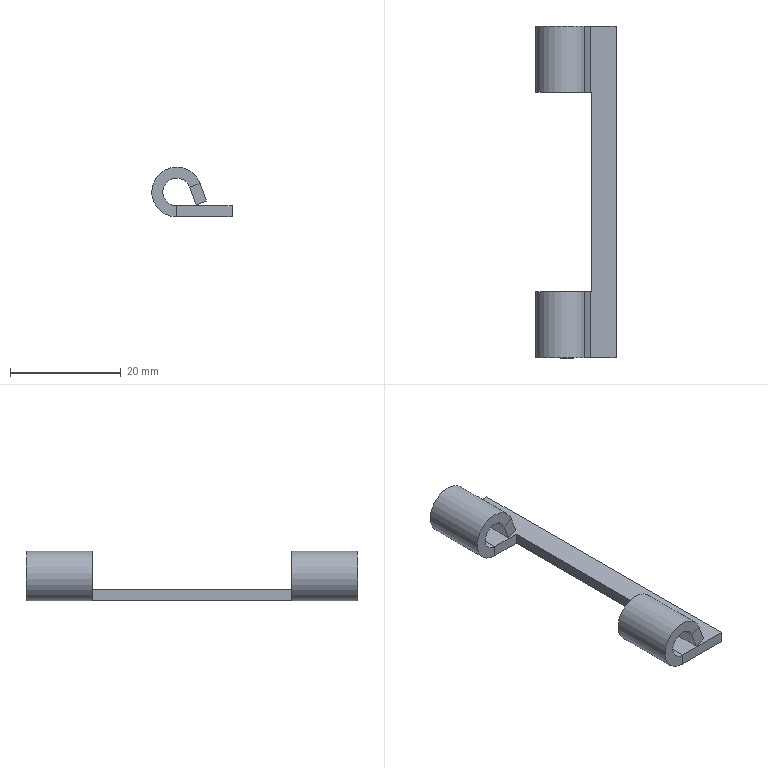Part | SolidWorks | features FlatPattern 1, Hem 1, ICE 1, SMBaseFlange 1, SheetMetal 1 | 1 solid | 26 faces | box 14.5 x 60 x 9 mm | volume 1699 mm3 | plane 22 | cylinder 4 | commonest cylinder face diameters 5 x2 9 x2
STEP:
#1=CARTESIAN_POINT('',(-0.4008,-18.,3.355));
#2=VERTEX_POINT('',#1);
#3=CARTESIAN_POINT('',(0.752,-18.,0.1879));
#4=VERTEX_POINT('',#3);
#5=CARTESIAN_POINT('',(0.1756,-18.,1.771));
#6=DIRECTION('',(0.342,0.,-0.9397));
#7=VECTOR('',#6,1000.);
#8=LINE('',#5,#7);
#9=EDGE_CURVE('',#2,#4,#8,.T.);
#10=ORIENTED_EDGE('',*,*,#9,.F.);
#11=CARTESIAN_POINT('',(1.479,-18.,4.039));
#12=VERTEX_POINT('',#11);
#13=CARTESIAN_POINT('',(-0.4008,-18.,3.355));
#14=DIRECTION('',(0.9397,0.,0.342));
#15=VECTOR('',#14,1000.);
#16=LINE('',#13,#15);
#17=EDGE_CURVE('',#2,#12,#16,.T.);
#18=ORIENTED_EDGE('',*,*,#17,.T.);
#19=CARTESIAN_POINT('',(2.631,-18.,0.872));
#20=VERTEX_POINT('',#19);
#21=CARTESIAN_POINT('',(2.055,-18.,2.456));
#22=DIRECTION('',(0.342,0.,-0.9397));
#23=VECTOR('',#22,1000.);
#24=LINE('',#21,#23);
#25=EDGE_CURVE('',#12,#20,#24,.T.);
#26=ORIENTED_EDGE('',*,*,#25,.T.);
#27=CARTESIAN_POINT('',(2.631,-18.,0.872));
#28=DIRECTION('',(-0.9397,0.,-0.342));
#29=VECTOR('',#28,1000.);
#30=LINE('',#27,#29);
#31=EDGE_CURVE('',#20,#4,#30,.T.);
#32=ORIENTED_EDGE('',*,*,#31,.T.);
#33=EDGE_LOOP('',(#10,#18,#26,#32));
#34=FACE_OUTER_BOUND('',#33,.T.);
#35=CARTESIAN_POINT('',(-8.25,-18.,7.));
#36=DIRECTION('',(0.,-1.,0.));
#37=DIRECTION('',(0.,0.,-1.));
#38=AXIS2_PLACEMENT_3D('',#35,#36,#37);
#39=PLANE('',#38);
#40=ADVANCED_FACE('',(#34),#39,.F.);
#41=CARTESIAN_POINT('',(2.75,-18.,-2.));
#42=VERTEX_POINT('',#41);
#43=CARTESIAN_POINT('',(-2.75,-18.,-2.));
#44=VERTEX_POINT('',#43);
#45=CARTESIAN_POINT('',(-8.25,-18.,-2.));
#46=DIRECTION('',(-1.,0.,0.));
#47=VECTOR('',#46,1000.);
#48=LINE('',#45,#47);
#49=EDGE_CURVE('',#42,#44,#48,.T.);
#50=ORIENTED_EDGE('',*,*,#49,.T.);
#51=CARTESIAN_POINT('',(-2.75,-18.,0.));
#52=VERTEX_POINT('',#51);
#53=CARTESIAN_POINT('',(-2.75,-18.,-2.));
#54=DIRECTION('',(0.,0.,1.));
#55=VECTOR('',#54,1000.);
#56=LINE('',#53,#55);
#57=EDGE_CURVE('',#44,#52,#56,.T.);
#58=ORIENTED_EDGE('',*,*,#57,.T.);
#59=CARTESIAN_POINT('',(2.75,-18.,0.));
#60=VERTEX_POINT('',#59);
#61=CARTESIAN_POINT('',(0.,-18.,0.));
#62=DIRECTION('',(-1.,0.,0.));
#63=VECTOR('',#62,1000.);
#64=LINE('',#61,#63);
#65=EDGE_CURVE('',#60,#52,#64,.T.);
#66=ORIENTED_EDGE('',*,*,#65,.F.);
#67=CARTESIAN_POINT('',(2.75,-18.,7.));
#68=DIRECTION('',(0.,0.,-1.));
#69=VECTOR('',#68,1000.);
#70=LINE('',#67,#69);
#71=EDGE_CURVE('',#60,#42,#70,.T.);
#72=ORIENTED_EDGE('',*,*,#71,.T.);
#73=EDGE_LOOP('',(#50,#58,#66,#72));
#74=FACE_OUTER_BOUND('',#73,.T.);
#75=CARTESIAN_POINT('',(-8.25,-18.,7.));
#76=DIRECTION('',(0.,-1.,0.));
#77=DIRECTION('',(0.,0.,-1.));
#78=AXIS2_PLACEMENT_3D('',#75,#76,#77);
#79=PLANE('',#78);
#80=ADVANCED_FACE('',(#74),#79,.F.);
#81=CARTESIAN_POINT('',(2.631,18.,0.872));
#82=VERTEX_POINT('',#81);
#83=CARTESIAN_POINT('',(1.479,18.,4.039));
#84=VERTEX_POINT('',#83);
#85=CARTESIAN_POINT('',(2.055,18.,2.456));
#86=DIRECTION('',(-0.342,0.,0.9397));
#87=VECTOR('',#86,1000.);
#88=LINE('',#85,#87);
#89=EDGE_CURVE('',#82,#84,#88,.T.);
#90=ORIENTED_EDGE('',*,*,#89,.T.);
#91=CARTESIAN_POINT('',(-0.4008,18.,3.355));
#92=VERTEX_POINT('',#91);
#93=CARTESIAN_POINT('',(1.479,18.,4.039));
#94=DIRECTION('',(-0.9397,0.,-0.342));
#95=VECTOR('',#94,1000.);
#96=LINE('',#93,#95);
#97=EDGE_CURVE('',#84,#92,#96,.T.);
#98=ORIENTED_EDGE('',*,*,#97,.T.);
#99=CARTESIAN_POINT('',(0.752,18.,0.1879));
#100=VERTEX_POINT('',#99);
#101=CARTESIAN_POINT('',(0.1756,18.,1.771));
#102=DIRECTION('',(-0.342,0.,0.9397));
#103=VECTOR('',#102,1000.);
#104=LINE('',#101,#103);
#105=EDGE_CURVE('',#100,#92,#104,.T.);
#106=ORIENTED_EDGE('',*,*,#105,.F.);
#107=CARTESIAN_POINT('',(2.631,18.,0.872));
#108=DIRECTION('',(0.9397,0.,0.342));
#109=VECTOR('',#108,1000.);
#110=LINE('',#107,#109);
#111=EDGE_CURVE('',#100,#82,#110,.T.);
#112=ORIENTED_EDGE('',*,*,#111,.T.);
#113=EDGE_LOOP('',(#90,#98,#106,#112));
#114=FACE_OUTER_BOUND('',#113,.T.);
#115=CARTESIAN_POINT('',(-8.25,18.,7.));
#116=DIRECTION('',(0.,1.,0.));
#117=DIRECTION('',(-1.,0.,0.));
#118=AXIS2_PLACEMENT_3D('',#115,#116,#117);
#119=PLANE('',#118);
#120=ADVANCED_FACE('',(#114),#119,.F.);
#121=CARTESIAN_POINT('',(-2.75,18.,0.));
#122=VERTEX_POINT('',#121);
#123=CARTESIAN_POINT('',(2.75,18.,0.));
#124=VERTEX_POINT('',#123);
#125=CARTESIAN_POINT('',(0.,18.,0.));
#126=DIRECTION('',(1.,0.,0.));
#127=VECTOR('',#126,1000.);
#128=LINE('',#125,#127);
#129=EDGE_CURVE('',#122,#124,#128,.T.);
#130=ORIENTED_EDGE('',*,*,#129,.F.);
#131=CARTESIAN_POINT('',(-2.75,18.,-2.));
#132=VERTEX_POINT('',#131);
#133=CARTESIAN_POINT('',(-2.75,18.,0.));
#134=DIRECTION('',(0.,0.,-1.));
#135=VECTOR('',#134,1000.);
#136=LINE('',#133,#135);
#137=EDGE_CURVE('',#122,#132,#136,.T.);
#138=ORIENTED_EDGE('',*,*,#137,.T.);
#139=CARTESIAN_POINT('',(2.75,18.,-2.));
#140=VERTEX_POINT('',#139);
#141=CARTESIAN_POINT('',(-8.25,18.,-2.));
#142=DIRECTION('',(1.,0.,0.));
#143=VECTOR('',#142,1000.);
#144=LINE('',#141,#143);
#145=EDGE_CURVE('',#132,#140,#144,.T.);
#146=ORIENTED_EDGE('',*,*,#145,.T.);
#147=CARTESIAN_POINT('',(2.75,18.,7.));
#148=DIRECTION('',(0.,0.,-1.));
#149=VECTOR('',#148,1000.);
#150=LINE('',#147,#149);
#151=EDGE_CURVE('',#124,#140,#150,.T.);
#152=ORIENTED_EDGE('',*,*,#151,.F.);
#153=EDGE_LOOP('',(#130,#138,#146,#152));
#154=FACE_OUTER_BOUND('',#153,.T.);
#155=CARTESIAN_POINT('',(-8.25,18.,7.));
#156=DIRECTION('',(0.,1.,0.));
#157=DIRECTION('',(-1.,0.,0.));
#158=AXIS2_PLACEMENT_3D('',#155,#156,#157);
#159=PLANE('',#158);
#160=ADVANCED_FACE('',(#154),#159,.F.);
#161=ORIENTED_EDGE('',*,*,#111,.F.);
#162=CARTESIAN_POINT('',(0.752,30.,0.1879));
#163=VERTEX_POINT('',#162);
#164=CARTESIAN_POINT('',(0.752,0.,0.1879));
#165=DIRECTION('',(0.,-1.,0.));
#166=VECTOR('',#165,1000.);
#167=LINE('',#164,#166);
#168=EDGE_CURVE('',#163,#100,#167,.T.);
#169=ORIENTED_EDGE('',*,*,#168,.F.);
#170=CARTESIAN_POINT('',(2.631,30.,0.872));
#171=VERTEX_POINT('',#170);
#172=CARTESIAN_POINT('',(2.631,30.,0.872));
#173=DIRECTION('',(0.9397,0.,0.342));
#174=VECTOR('',#173,1000.);
#175=LINE('',#172,#174);
#176=EDGE_CURVE('',#163,#171,#175,.T.);
#177=ORIENTED_EDGE('',*,*,#176,.T.);
#178=CARTESIAN_POINT('',(2.631,0.,0.872));
#179=DIRECTION('',(0.,-1.,0.));
#180=VECTOR('',#179,1000.);
#181=LINE('',#178,#180);
#182=EDGE_CURVE('',#171,#82,#181,.T.);
#183=ORIENTED_EDGE('',*,*,#182,.T.);
#184=EDGE_LOOP('',(#161,#169,#177,#183));
#185=FACE_OUTER_BOUND('',#184,.T.);
#186=CARTESIAN_POINT('',(2.631,0.,0.872));
#187=DIRECTION('',(-0.342,0.,0.9397));
#188=DIRECTION('',(0.,-1.,0.));
#189=AXIS2_PLACEMENT_3D('',#186,#187,#188);
#190=PLANE('',#189);
#191=ADVANCED_FACE('',(#185),#190,.F.);
#192=ORIENTED_EDGE('',*,*,#89,.F.);
#193=ORIENTED_EDGE('',*,*,#182,.F.);
#194=CARTESIAN_POINT('',(1.479,30.,4.039));
#195=VERTEX_POINT('',#194);
#196=CARTESIAN_POINT('',(2.055,30.,2.456));
#197=DIRECTION('',(0.342,0.,-0.9397));
#198=VECTOR('',#197,1000.);
#199=LINE('',#196,#198);
#200=EDGE_CURVE('',#195,#171,#199,.T.);
#201=ORIENTED_EDGE('',*,*,#200,.F.);
#202=CARTESIAN_POINT('',(1.479,0.,4.039));
#203=DIRECTION('',(0.,1.,0.));
#204=VECTOR('',#203,1000.);
#205=LINE('',#202,#204);
#206=EDGE_CURVE('',#84,#195,#205,.T.);
#207=ORIENTED_EDGE('',*,*,#206,.F.);
#208=EDGE_LOOP('',(#192,#193,#201,#207));
#209=FACE_OUTER_BOUND('',#208,.T.);
#210=CARTESIAN_POINT('',(2.055,0.,2.456));
#211=DIRECTION('',(0.9397,0.,0.342));
#212=DIRECTION('',(0.342,0.,-0.9397));
#213=AXIS2_PLACEMENT_3D('',#210,#211,#212);
#214=PLANE('',#213);
#215=ADVANCED_FACE('',(#209),#214,.T.);
#216=ORIENTED_EDGE('',*,*,#168,.T.);
#217=ORIENTED_EDGE('',*,*,#105,.T.);
#218=CARTESIAN_POINT('',(-0.4008,30.,3.355));
#219=VERTEX_POINT('',#218);
#220=CARTESIAN_POINT('',(-0.4008,0.,3.355));
#221=DIRECTION('',(0.,1.,0.));
#222=VECTOR('',#221,1000.);
#223=LINE('',#220,#222);
#224=EDGE_CURVE('',#92,#219,#223,.T.);
#225=ORIENTED_EDGE('',*,*,#224,.T.);
#226=CARTESIAN_POINT('',(0.1756,30.,1.771));
#227=DIRECTION('',(0.342,0.,-0.9397));
#228=VECTOR('',#227,1000.);
#229=LINE('',#226,#228);
#230=EDGE_CURVE('',#219,#163,#229,.T.);
#231=ORIENTED_EDGE('',*,*,#230,.T.);
#232=EDGE_LOOP('',(#216,#217,#225,#231));
#233=FACE_OUTER_BOUND('',#232,.T.);
#234=CARTESIAN_POINT('',(0.1756,0.,1.771));
#235=DIRECTION('',(0.9397,0.,0.342));
#236=DIRECTION('',(0.342,0.,-0.9397));
#237=AXIS2_PLACEMENT_3D('',#234,#235,#236);
#238=PLANE('',#237);
#239=ADVANCED_FACE('',(#233),#238,.F.);
#240=CARTESIAN_POINT('',(-2.75,-18.,2.5));
#241=DIRECTION('',(0.,1.,0.));
#242=DIRECTION('',(0.,0.,-1.));
#243=AXIS2_PLACEMENT_3D('',#240,#241,#242);
#244=CIRCLE('',#243,4.5);
#245=EDGE_CURVE('',#44,#12,#244,.T.);
#246=ORIENTED_EDGE('',*,*,#245,.F.);
#247=CARTESIAN_POINT('',(-2.75,-30.,-2.));
#248=VERTEX_POINT('',#247);
#249=CARTESIAN_POINT('',(-2.75,-30.,-2.));
#250=DIRECTION('',(0.,1.,0.));
#251=VECTOR('',#250,1000.);
#252=LINE('',#249,#251);
#253=EDGE_CURVE('',#248,#44,#252,.T.);
#254=ORIENTED_EDGE('',*,*,#253,.F.);
#255=CARTESIAN_POINT('',(1.479,-30.,4.039));
#256=VERTEX_POINT('',#255);
#257=CARTESIAN_POINT('',(-2.75,-30.,2.5));
#258=DIRECTION('',(0.,-1.,0.));
#259=DIRECTION('',(0.,0.,-1.));
#260=AXIS2_PLACEMENT_3D('',#257,#258,#259);
#261=CIRCLE('',#260,4.5);
#262=EDGE_CURVE('',#256,#248,#261,.T.);
#263=ORIENTED_EDGE('',*,*,#262,.F.);
#264=CARTESIAN_POINT('',(1.479,0.,4.039));
#265=DIRECTION('',(0.,1.,0.));
#266=VECTOR('',#265,1000.);
#267=LINE('',#264,#266);
#268=EDGE_CURVE('',#256,#12,#267,.T.);
#269=ORIENTED_EDGE('',*,*,#268,.T.);
#270=EDGE_LOOP('',(#246,#254,#263,#269));
#271=FACE_OUTER_BOUND('',#270,.T.);
#272=CARTESIAN_POINT('',(-2.75,-30.,2.5));
#273=DIRECTION('',(0.,-1.,0.));
#274=DIRECTION('',(0.9397,0.,0.342));
#275=AXIS2_PLACEMENT_3D('',#272,#273,#274);
#276=CYLINDRICAL_SURFACE('',#275,4.5);
#277=ADVANCED_FACE('',(#271),#276,.T.);
#278=ORIENTED_EDGE('',*,*,#224,.F.);
#279=CARTESIAN_POINT('',(-2.75,18.,2.5));
#280=DIRECTION('',(0.,-1.,0.));
#281=DIRECTION('',(-1.,0.,0.));
#282=AXIS2_PLACEMENT_3D('',#279,#280,#281);
#283=CIRCLE('',#282,2.5);
#284=EDGE_CURVE('',#92,#122,#283,.T.);
#285=ORIENTED_EDGE('',*,*,#284,.T.);
#286=CARTESIAN_POINT('',(-2.75,30.,0.));
#287=VERTEX_POINT('',#286);
#288=CARTESIAN_POINT('',(-2.75,-30.,0.));
#289=DIRECTION('',(0.,1.,0.));
#290=VECTOR('',#289,1000.);
#291=LINE('',#288,#290);
#292=EDGE_CURVE('',#122,#287,#291,.T.);
#293=ORIENTED_EDGE('',*,*,#292,.T.);
#294=CARTESIAN_POINT('',(-2.75,30.,2.5));
#295=DIRECTION('',(0.,1.,0.));
#296=DIRECTION('',(0.,0.,-1.));
#297=AXIS2_PLACEMENT_3D('',#294,#295,#296);
#298=CIRCLE('',#297,2.5);
#299=EDGE_CURVE('',#287,#219,#298,.T.);
#300=ORIENTED_EDGE('',*,*,#299,.T.);
#301=EDGE_LOOP('',(#278,#285,#293,#300));
#302=FACE_OUTER_BOUND('',#301,.T.);
#303=CARTESIAN_POINT('',(-2.75,-30.,2.5));
#304=DIRECTION('',(0.,-1.,0.));
#305=DIRECTION('',(0.9397,0.,0.342));
#306=AXIS2_PLACEMENT_3D('',#303,#304,#305);
#307=CYLINDRICAL_SURFACE('',#306,2.5);
#308=ADVANCED_FACE('',(#302),#307,.F.);
#309=CARTESIAN_POINT('',(-2.75,-30.,0.));
#310=VERTEX_POINT('',#309);
#311=CARTESIAN_POINT('',(7.25,-30.,0.));
#312=VERTEX_POINT('',#311);
#313=CARTESIAN_POINT('',(-7.25,-30.,0.));
#314=DIRECTION('',(1.,0.,0.));
#315=VECTOR('',#314,1000.);
#316=LINE('',#313,#315);
#317=EDGE_CURVE('',#310,#312,#316,.T.);
#318=ORIENTED_EDGE('',*,*,#317,.F.);
#319=CARTESIAN_POINT('',(-2.75,-30.,0.));
#320=DIRECTION('',(0.,0.,-1.));
#321=VECTOR('',#320,1000.);
#322=LINE('',#319,#321);
#323=EDGE_CURVE('',#310,#248,#322,.T.);
#324=ORIENTED_EDGE('',*,*,#323,.T.);
#325=CARTESIAN_POINT('',(7.25,-30.,-2.));
#326=VERTEX_POINT('',#325);
#327=CARTESIAN_POINT('',(-7.25,-30.,-2.));
#328=DIRECTION('',(1.,0.,0.));
#329=VECTOR('',#328,1000.);
#330=LINE('',#327,#329);
#331=EDGE_CURVE('',#248,#326,#330,.T.);
#332=ORIENTED_EDGE('',*,*,#331,.T.);
#333=CARTESIAN_POINT('',(7.25,-30.,-2.));
#334=DIRECTION('',(0.,0.,1.));
#335=VECTOR('',#334,1000.);
#336=LINE('',#333,#335);
#337=EDGE_CURVE('',#326,#312,#336,.T.);
#338=ORIENTED_EDGE('',*,*,#337,.T.);
#339=EDGE_LOOP('',(#318,#324,#332,#338));
#340=FACE_OUTER_BOUND('',#339,.T.);
#341=CARTESIAN_POINT('',(-7.25,-30.,-2.));
#342=DIRECTION('',(0.,-1.,0.));
#343=DIRECTION('',(0.,0.,-1.));
#344=AXIS2_PLACEMENT_3D('',#341,#342,#343);
#345=PLANE('',#344);
#346=ADVANCED_FACE('',(#340),#345,.T.);
#347=CARTESIAN_POINT('',(7.25,30.,0.));
#348=VERTEX_POINT('',#347);
#349=CARTESIAN_POINT('',(7.25,-30.,0.));
#350=DIRECTION('',(0.,1.,0.));
#351=VECTOR('',#350,1000.);
#352=LINE('',#349,#351);
#353=EDGE_CURVE('',#312,#348,#352,.T.);
#354=ORIENTED_EDGE('',*,*,#353,.F.);
#355=ORIENTED_EDGE('',*,*,#337,.F.);
#356=CARTESIAN_POINT('',(7.25,30.,-2.));
#357=VERTEX_POINT('',#356);
#358=CARTESIAN_POINT('',(7.25,-30.,-2.));
#359=DIRECTION('',(0.,1.,0.));
#360=VECTOR('',#359,1000.);
#361=LINE('',#358,#360);
#362=EDGE_CURVE('',#326,#357,#361,.T.);
#363=ORIENTED_EDGE('',*,*,#362,.T.);
#364=CARTESIAN_POINT('',(7.25,30.,-2.));
#365=DIRECTION('',(0.,0.,1.));
#366=VECTOR('',#365,1000.);
#367=LINE('',#364,#366);
#368=EDGE_CURVE('',#357,#348,#367,.T.);
#369=ORIENTED_EDGE('',*,*,#368,.T.);
#370=EDGE_LOOP('',(#354,#355,#363,#369));
#371=FACE_OUTER_BOUND('',#370,.T.);
#372=CARTESIAN_POINT('',(7.25,-30.,-2.));
#373=DIRECTION('',(1.,0.,0.));
#374=DIRECTION('',(0.,0.,-1.));
#375=AXIS2_PLACEMENT_3D('',#372,#373,#374);
#376=PLANE('',#375);
#377=ADVANCED_FACE('',(#371),#376,.T.);
#378=CARTESIAN_POINT('',(-2.75,30.,-2.));
#379=VERTEX_POINT('',#378);
#380=CARTESIAN_POINT('',(-2.75,30.,0.));
#381=DIRECTION('',(0.,0.,-1.));
#382=VECTOR('',#381,1000.);
#383=LINE('',#380,#382);
#384=EDGE_CURVE('',#287,#379,#383,.T.);
#385=ORIENTED_EDGE('',*,*,#384,.F.);
#386=CARTESIAN_POINT('',(-7.25,30.,0.));
#387=DIRECTION('',(-1.,0.,0.));
#388=VECTOR('',#387,1000.);
#389=LINE('',#386,#388);
#390=EDGE_CURVE('',#348,#287,#389,.T.);
#391=ORIENTED_EDGE('',*,*,#390,.F.);
#392=ORIENTED_EDGE('',*,*,#368,.F.);
#393=CARTESIAN_POINT('',(-7.25,30.,-2.));
#394=DIRECTION('',(-1.,0.,0.));
#395=VECTOR('',#394,1000.);
#396=LINE('',#393,#395);
#397=EDGE_CURVE('',#357,#379,#396,.T.);
#398=ORIENTED_EDGE('',*,*,#397,.T.);
#399=EDGE_LOOP('',(#385,#391,#392,#398));
#400=FACE_OUTER_BOUND('',#399,.T.);
#401=CARTESIAN_POINT('',(-7.25,30.,-2.));
#402=DIRECTION('',(0.,1.,0.));
#403=DIRECTION('',(0.,0.,1.));
#404=AXIS2_PLACEMENT_3D('',#401,#402,#403);
#405=PLANE('',#404);
#406=ADVANCED_FACE('',(#400),#405,.T.);
#407=ORIENTED_EDGE('',*,*,#145,.F.);
#408=CARTESIAN_POINT('',(-2.75,-30.,-2.));
#409=DIRECTION('',(0.,1.,0.));
#410=VECTOR('',#409,1000.);
#411=LINE('',#408,#410);
#412=EDGE_CURVE('',#132,#379,#411,.T.);
#413=ORIENTED_EDGE('',*,*,#412,.T.);
#414=ORIENTED_EDGE('',*,*,#397,.F.);
#415=ORIENTED_EDGE('',*,*,#362,.F.);
#416=ORIENTED_EDGE('',*,*,#331,.F.);
#417=ORIENTED_EDGE('',*,*,#253,.T.);
#418=ORIENTED_EDGE('',*,*,#49,.F.);
#419=CARTESIAN_POINT('',(2.75,-18.,-2.));
#420=DIRECTION('',(0.,-1.,0.));
#421=VECTOR('',#420,1000.);
#422=LINE('',#419,#421);
#423=EDGE_CURVE('',#140,#42,#422,.T.);
#424=ORIENTED_EDGE('',*,*,#423,.F.);
#425=EDGE_LOOP('',(#407,#413,#414,#415,#416,#417,#418,#424));
#426=FACE_OUTER_BOUND('',#425,.T.);
#427=CARTESIAN_POINT('',(0.,0.,-2.));
#428=DIRECTION('',(0.,0.,-1.));
#429=DIRECTION('',(-1.,0.,0.));
#430=AXIS2_PLACEMENT_3D('',#427,#428,#429);
#431=PLANE('',#430);
#432=ADVANCED_FACE('',(#426),#431,.T.);
#433=ORIENTED_EDGE('',*,*,#292,.F.);
#434=ORIENTED_EDGE('',*,*,#129,.T.);
#435=CARTESIAN_POINT('',(2.75,0.,0.));
#436=DIRECTION('',(0.,-1.,0.));
#437=VECTOR('',#436,1000.);
#438=LINE('',#435,#437);
#439=EDGE_CURVE('',#124,#60,#438,.T.);
#440=ORIENTED_EDGE('',*,*,#439,.T.);
#441=ORIENTED_EDGE('',*,*,#65,.T.);
#442=CARTESIAN_POINT('',(-2.75,-30.,0.));
#443=DIRECTION('',(0.,1.,0.));
#444=VECTOR('',#443,1000.);
#445=LINE('',#442,#444);
#446=EDGE_CURVE('',#310,#52,#445,.T.);
#447=ORIENTED_EDGE('',*,*,#446,.F.);
#448=ORIENTED_EDGE('',*,*,#317,.T.);
#449=ORIENTED_EDGE('',*,*,#353,.T.);
#450=ORIENTED_EDGE('',*,*,#390,.T.);
#451=EDGE_LOOP('',(#433,#434,#440,#441,#447,#448,#449,#450));
#452=FACE_OUTER_BOUND('',#451,.T.);
#453=CARTESIAN_POINT('',(0.,0.,0.));
#454=DIRECTION('',(0.,0.,-1.));
#455=DIRECTION('',(-1.,0.,0.));
#456=AXIS2_PLACEMENT_3D('',#453,#454,#455);
#457=PLANE('',#456);
#458=ADVANCED_FACE('',(#452),#457,.F.);
#459=CARTESIAN_POINT('',(-0.4008,-30.,3.355));
#460=VERTEX_POINT('',#459);
#461=CARTESIAN_POINT('',(1.479,-30.,4.039));
#462=DIRECTION('',(0.9397,0.,0.342));
#463=VECTOR('',#462,1000.);
#464=LINE('',#461,#463);
#465=EDGE_CURVE('',#460,#256,#464,.T.);
#466=ORIENTED_EDGE('',*,*,#465,.F.);
#467=CARTESIAN_POINT('',(0.752,-30.,0.1879));
#468=VERTEX_POINT('',#467);
#469=CARTESIAN_POINT('',(0.1756,-30.,1.771));
#470=DIRECTION('',(-0.342,0.,0.9397));
#471=VECTOR('',#470,1000.);
#472=LINE('',#469,#471);
#473=EDGE_CURVE('',#468,#460,#472,.T.);
#474=ORIENTED_EDGE('',*,*,#473,.F.);
#475=CARTESIAN_POINT('',(2.631,-30.,0.872));
#476=VERTEX_POINT('',#475);
#477=CARTESIAN_POINT('',(2.631,-30.,0.872));
#478=DIRECTION('',(0.9397,0.,0.342));
#479=VECTOR('',#478,1000.);
#480=LINE('',#477,#479);
#481=EDGE_CURVE('',#468,#476,#480,.T.);
#482=ORIENTED_EDGE('',*,*,#481,.T.);
#483=CARTESIAN_POINT('',(2.055,-30.,2.456));
#484=DIRECTION('',(-0.342,0.,0.9397));
#485=VECTOR('',#484,1000.);
#486=LINE('',#483,#485);
#487=EDGE_CURVE('',#476,#256,#486,.T.);
#488=ORIENTED_EDGE('',*,*,#487,.T.);
#489=EDGE_LOOP('',(#466,#474,#482,#488));
#490=FACE_OUTER_BOUND('',#489,.T.);
#491=CARTESIAN_POINT('',(2.055,-30.,2.456));
#492=DIRECTION('',(0.,1.,0.));
#493=DIRECTION('',(-0.342,0.,0.9397));
#494=AXIS2_PLACEMENT_3D('',#491,#492,#493);
#495=PLANE('',#494);
#496=ADVANCED_FACE('',(#490),#495,.F.);
#497=ORIENTED_EDGE('',*,*,#31,.F.);
#498=CARTESIAN_POINT('',(2.631,0.,0.872));
#499=DIRECTION('',(0.,-1.,0.));
#500=VECTOR('',#499,1000.);
#501=LINE('',#498,#500);
#502=EDGE_CURVE('',#20,#476,#501,.T.);
#503=ORIENTED_EDGE('',*,*,#502,.T.);
#504=ORIENTED_EDGE('',*,*,#481,.F.);
#505=CARTESIAN_POINT('',(0.752,0.,0.1879));
#506=DIRECTION('',(0.,-1.,0.));
#507=VECTOR('',#506,1000.);
#508=LINE('',#505,#507);
#509=EDGE_CURVE('',#4,#468,#508,.T.);
#510=ORIENTED_EDGE('',*,*,#509,.F.);
#511=EDGE_LOOP('',(#497,#503,#504,#510));
#512=FACE_OUTER_BOUND('',#511,.T.);
#513=CARTESIAN_POINT('',(2.631,0.,0.872));
#514=DIRECTION('',(-0.342,0.,0.9397));
#515=DIRECTION('',(0.,-1.,0.));
#516=AXIS2_PLACEMENT_3D('',#513,#514,#515);
#517=PLANE('',#516);
#518=ADVANCED_FACE('',(#512),#517,.F.);
#519=ORIENTED_EDGE('',*,*,#230,.F.);
#520=CARTESIAN_POINT('',(1.479,30.,4.039));
#521=DIRECTION('',(0.9397,0.,0.342));
#522=VECTOR('',#521,1000.);
#523=LINE('',#520,#522);
#524=EDGE_CURVE('',#219,#195,#523,.T.);
#525=ORIENTED_EDGE('',*,*,#524,.T.);
#526=ORIENTED_EDGE('',*,*,#200,.T.);
#527=ORIENTED_EDGE('',*,*,#176,.F.);
#528=EDGE_LOOP('',(#519,#525,#526,#527));
#529=FACE_OUTER_BOUND('',#528,.T.);
#530=CARTESIAN_POINT('',(2.055,30.,2.456));
#531=DIRECTION('',(0.,-1.,0.));
#532=DIRECTION('',(0.342,0.,-0.9397));
#533=AXIS2_PLACEMENT_3D('',#530,#531,#532);
#534=PLANE('',#533);
#535=ADVANCED_FACE('',(#529),#534,.F.);
#536=ORIENTED_EDGE('',*,*,#25,.F.);
#537=ORIENTED_EDGE('',*,*,#268,.F.);
#538=ORIENTED_EDGE('',*,*,#487,.F.);
#539=ORIENTED_EDGE('',*,*,#502,.F.);
#540=EDGE_LOOP('',(#536,#537,#538,#539));
#541=FACE_OUTER_BOUND('',#540,.T.);
#542=CARTESIAN_POINT('',(2.055,0.,2.456));
#543=DIRECTION('',(0.9397,0.,0.342));
#544=DIRECTION('',(0.342,0.,-0.9397));
#545=AXIS2_PLACEMENT_3D('',#542,#543,#544);
#546=PLANE('',#545);
#547=ADVANCED_FACE('',(#541),#546,.T.);
#548=CARTESIAN_POINT('',(-0.4008,0.,3.355));
#549=DIRECTION('',(0.,1.,0.));
#550=VECTOR('',#549,1000.);
#551=LINE('',#548,#550);
#552=EDGE_CURVE('',#460,#2,#551,.T.);
#553=ORIENTED_EDGE('',*,*,#552,.T.);
#554=ORIENTED_EDGE('',*,*,#9,.T.);
#555=ORIENTED_EDGE('',*,*,#509,.T.);
#556=ORIENTED_EDGE('',*,*,#473,.T.);
#557=EDGE_LOOP('',(#553,#554,#555,#556));
#558=FACE_OUTER_BOUND('',#557,.T.);
#559=CARTESIAN_POINT('',(0.1756,0.,1.771));
#560=DIRECTION('',(0.9397,0.,0.342));
#561=DIRECTION('',(0.342,0.,-0.9397));
#562=AXIS2_PLACEMENT_3D('',#559,#560,#561);
#563=PLANE('',#562);
#564=ADVANCED_FACE('',(#558),#563,.F.);
#565=ORIENTED_EDGE('',*,*,#524,.F.);
#566=ORIENTED_EDGE('',*,*,#299,.F.);
#567=ORIENTED_EDGE('',*,*,#384,.T.);
#568=CARTESIAN_POINT('',(-2.75,30.,2.5));
#569=DIRECTION('',(0.,1.,0.));
#570=DIRECTION('',(0.,0.,-1.));
#571=AXIS2_PLACEMENT_3D('',#568,#569,#570);
#572=CIRCLE('',#571,4.5);
#573=EDGE_CURVE('',#379,#195,#572,.T.);
#574=ORIENTED_EDGE('',*,*,#573,.T.);
#575=EDGE_LOOP('',(#565,#566,#567,#574));
#576=FACE_OUTER_BOUND('',#575,.T.);
#577=CARTESIAN_POINT('',(-2.75,30.,2.5));
#578=DIRECTION('',(0.,1.,0.));
#579=DIRECTION('',(0.,0.,1.));
#580=AXIS2_PLACEMENT_3D('',#577,#578,#579);
#581=PLANE('',#580);
#582=ADVANCED_FACE('',(#576),#581,.T.);
#583=CARTESIAN_POINT('',(-2.75,-30.,2.5));
#584=DIRECTION('',(0.,-1.,0.));
#585=DIRECTION('',(0.,0.,-1.));
#586=AXIS2_PLACEMENT_3D('',#583,#584,#585);
#587=CIRCLE('',#586,2.5);
#588=EDGE_CURVE('',#460,#310,#587,.T.);
#589=ORIENTED_EDGE('',*,*,#588,.F.);
#590=ORIENTED_EDGE('',*,*,#465,.T.);
#591=ORIENTED_EDGE('',*,*,#262,.T.);
#592=ORIENTED_EDGE('',*,*,#323,.F.);
#593=EDGE_LOOP('',(#589,#590,#591,#592));
#594=FACE_OUTER_BOUND('',#593,.T.);
#595=CARTESIAN_POINT('',(-2.75,-30.,2.5));
#596=DIRECTION('',(0.,1.,0.));
#597=DIRECTION('',(0.,0.,1.));
#598=AXIS2_PLACEMENT_3D('',#595,#596,#597);
#599=PLANE('',#598);
#600=ADVANCED_FACE('',(#594),#599,.F.);
#601=CARTESIAN_POINT('',(-2.75,18.,2.5));
#602=DIRECTION('',(0.,-1.,0.));
#603=DIRECTION('',(-1.,0.,0.));
#604=AXIS2_PLACEMENT_3D('',#601,#602,#603);
#605=CIRCLE('',#604,4.5);
#606=EDGE_CURVE('',#84,#132,#605,.T.);
#607=ORIENTED_EDGE('',*,*,#606,.F.);
#608=ORIENTED_EDGE('',*,*,#206,.T.);
#609=ORIENTED_EDGE('',*,*,#573,.F.);
#610=ORIENTED_EDGE('',*,*,#412,.F.);
#611=EDGE_LOOP('',(#607,#608,#609,#610));
#612=FACE_OUTER_BOUND('',#611,.T.);
#613=CARTESIAN_POINT('',(-2.75,-30.,2.5));
#614=DIRECTION('',(0.,-1.,0.));
#615=DIRECTION('',(0.9397,0.,0.342));
#616=AXIS2_PLACEMENT_3D('',#613,#614,#615);
#617=CYLINDRICAL_SURFACE('',#616,4.5);
#618=ADVANCED_FACE('',(#612),#617,.T.);
#619=ORIENTED_EDGE('',*,*,#446,.T.);
#620=CARTESIAN_POINT('',(-2.75,-18.,2.5));
#621=DIRECTION('',(0.,1.,0.));
#622=DIRECTION('',(0.,0.,-1.));
#623=AXIS2_PLACEMENT_3D('',#620,#621,#622);
#624=CIRCLE('',#623,2.5);
#625=EDGE_CURVE('',#52,#2,#624,.T.);
#626=ORIENTED_EDGE('',*,*,#625,.T.);
#627=ORIENTED_EDGE('',*,*,#552,.F.);
#628=ORIENTED_EDGE('',*,*,#588,.T.);
#629=EDGE_LOOP('',(#619,#626,#627,#628));
#630=FACE_OUTER_BOUND('',#629,.T.);
#631=CARTESIAN_POINT('',(-2.75,-30.,2.5));
#632=DIRECTION('',(0.,-1.,0.));
#633=DIRECTION('',(0.9397,0.,0.342));
#634=AXIS2_PLACEMENT_3D('',#631,#632,#633);
#635=CYLINDRICAL_SURFACE('',#634,2.5);
#636=ADVANCED_FACE('',(#630),#635,.F.);
#637=ORIENTED_EDGE('',*,*,#151,.T.);
#638=ORIENTED_EDGE('',*,*,#423,.T.);
#639=ORIENTED_EDGE('',*,*,#71,.F.);
#640=ORIENTED_EDGE('',*,*,#439,.F.);
#641=EDGE_LOOP('',(#637,#638,#639,#640));
#642=FACE_OUTER_BOUND('',#641,.T.);
#643=CARTESIAN_POINT('',(2.75,-18.,7.));
#644=DIRECTION('',(1.,0.,0.));
#645=DIRECTION('',(0.,1.,0.));
#646=AXIS2_PLACEMENT_3D('',#643,#644,#645);
#647=PLANE('',#646);
#648=ADVANCED_FACE('',(#642),#647,.F.);
#649=ORIENTED_EDGE('',*,*,#97,.F.);
#650=ORIENTED_EDGE('',*,*,#606,.T.);
#651=ORIENTED_EDGE('',*,*,#137,.F.);
#652=ORIENTED_EDGE('',*,*,#284,.F.);
#653=EDGE_LOOP('',(#649,#650,#651,#652));
#654=FACE_OUTER_BOUND('',#653,.T.);
#655=CARTESIAN_POINT('',(-8.25,18.,7.));
#656=DIRECTION('',(0.,1.,0.));
#657=DIRECTION('',(-1.,0.,0.));
#658=AXIS2_PLACEMENT_3D('',#655,#656,#657);
#659=PLANE('',#658);
#660=ADVANCED_FACE('',(#654),#659,.F.);
#661=ORIENTED_EDGE('',*,*,#17,.F.);
#662=ORIENTED_EDGE('',*,*,#625,.F.);
#663=ORIENTED_EDGE('',*,*,#57,.F.);
#664=ORIENTED_EDGE('',*,*,#245,.T.);
#665=EDGE_LOOP('',(#661,#662,#663,#664));
#666=FACE_OUTER_BOUND('',#665,.T.);
#667=CARTESIAN_POINT('',(-8.25,-18.,7.));
#668=DIRECTION('',(0.,-1.,0.));
#669=DIRECTION('',(0.,0.,-1.));
#670=AXIS2_PLACEMENT_3D('',#667,#668,#669);
#671=PLANE('',#670);
#672=ADVANCED_FACE('',(#666),#671,.F.);
#673=CLOSED_SHELL('',(#40,#80,#120,#160,#191,#215,#239,#277,#308,#346,#377,#406,#432,#458,#496,#518,#535,#547,#564,#582,#600,#618,#636,#648,#660,#672));
#674=MANIFOLD_SOLID_BREP('',#673);
#675=CARTESIAN_POINT('',(0.,0.,0.));
#676=DIRECTION('',(0.,0.,1.));
#677=DIRECTION('',(1.,0.,0.));
#678=AXIS2_PLACEMENT_3D('',#675,#676,#677);
#679=(LENGTH_UNIT()NAMED_UNIT(*)SI_UNIT(.MILLI.,.METRE.));
#680=UNCERTAINTY_MEASURE_WITH_UNIT(LENGTH_MEASURE(0.00001),#679,'','');
#681=(NAMED_UNIT(*)PLANE_ANGLE_UNIT()SI_UNIT($,.RADIAN.));
#682=(NAMED_UNIT(*)SI_UNIT($,.STERADIAN.)SOLID_ANGLE_UNIT());
#683=(GEOMETRIC_REPRESENTATION_CONTEXT(3)GLOBAL_UNCERTAINTY_ASSIGNED_CONTEXT((#680))GLOBAL_UNIT_ASSIGNED_CONTEXT((#679,#681,#682))REPRESENTATION_CONTEXT('',''));
#684=ADVANCED_BREP_SHAPE_REPRESENTATION('',(#674,#678),#683);